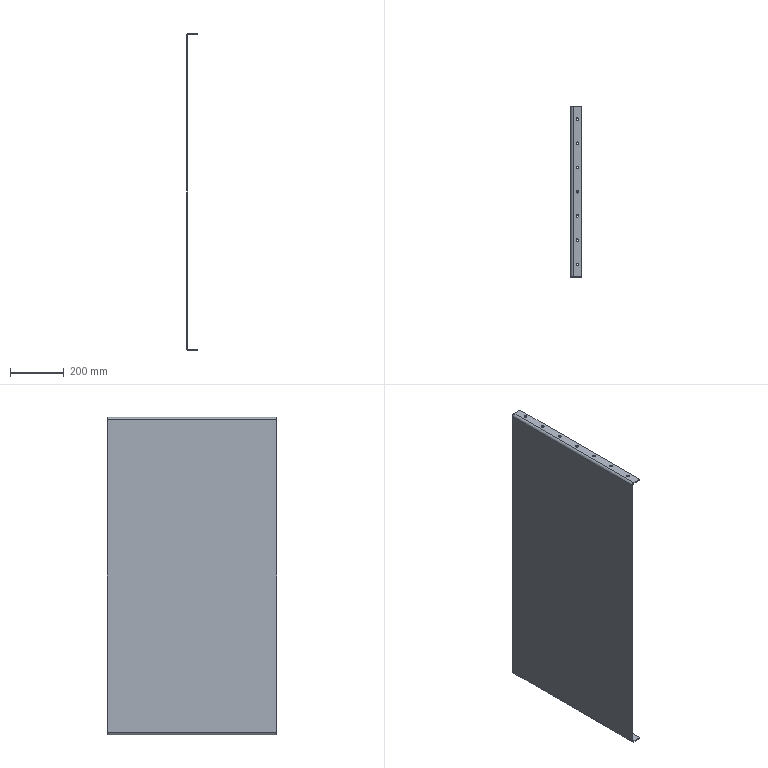Part | SolidWorks | features EdgeFlange 1, FlatPattern 1, HoleWzd 1, ICE 1, LPattern 1, SMBaseFlange 1, SheetMetal 1 | 1 solid | 50 faces | box 40 x 630 x 1180 mm | volume 3135499 mm3 | cylinder 32 | plane 18 | commonest cylinder face diameters 10 x30 18 x2
STEP:
#1=CARTESIAN_POINT('',(21.,40.,1180.));
#2=VERTEX_POINT('',#1);
#3=CARTESIAN_POINT('',(21.,50.,1180.));
#4=VERTEX_POINT('',#3);
#5=CARTESIAN_POINT('',(21.,45.,1180.));
#6=DIRECTION('',(0.,0.,-1.));
#7=DIRECTION('',(0.,1.,0.));
#8=AXIS2_PLACEMENT_3D('',#5,#6,#7);
#9=CIRCLE('',#8,5.);
#10=EDGE_CURVE('',#2,#4,#9,.T.);
#11=ORIENTED_EDGE('',*,*,#10,.F.);
#12=CARTESIAN_POINT('',(21.,40.,1176.));
#13=VERTEX_POINT('',#12);
#14=CARTESIAN_POINT('',(21.,40.,0.));
#15=DIRECTION('',(0.,0.,-1.));
#16=VECTOR('',#15,1000.);
#17=LINE('',#14,#16);
#18=EDGE_CURVE('',#2,#13,#17,.T.);
#19=ORIENTED_EDGE('',*,*,#18,.T.);
#20=CARTESIAN_POINT('',(21.,50.,1176.));
#21=VERTEX_POINT('',#20);
#22=CARTESIAN_POINT('',(21.,45.,1176.));
#23=DIRECTION('',(0.,0.,-1.));
#24=DIRECTION('',(-1.,0.,0.));
#25=AXIS2_PLACEMENT_3D('',#22,#23,#24);
#26=CIRCLE('',#25,5.);
#27=EDGE_CURVE('',#13,#21,#26,.T.);
#28=ORIENTED_EDGE('',*,*,#27,.T.);
#29=CARTESIAN_POINT('',(21.,50.,0.));
#30=DIRECTION('',(0.,0.,-1.));
#31=VECTOR('',#30,1000.);
#32=LINE('',#29,#31);
#33=EDGE_CURVE('',#4,#21,#32,.T.);
#34=ORIENTED_EDGE('',*,*,#33,.F.);
#35=EDGE_LOOP('',(#11,#19,#28,#34));
#36=FACE_OUTER_BOUND('',#35,.T.);
#37=CARTESIAN_POINT('',(21.,45.,0.));
#38=DIRECTION('',(0.,0.,-1.));
#39=DIRECTION('',(0.,1.,0.));
#40=AXIS2_PLACEMENT_3D('',#37,#38,#39);
#41=CYLINDRICAL_SURFACE('',#40,5.);
#42=ADVANCED_FACE('',(#36),#41,.F.);
#43=CARTESIAN_POINT('',(21.,130.,1180.));
#44=VERTEX_POINT('',#43);
#45=CARTESIAN_POINT('',(21.,140.,1180.));
#46=VERTEX_POINT('',#45);
#47=CARTESIAN_POINT('',(21.,135.,1180.));
#48=DIRECTION('',(0.,0.,-1.));
#49=DIRECTION('',(0.,1.,0.));
#50=AXIS2_PLACEMENT_3D('',#47,#48,#49);
#51=CIRCLE('',#50,5.);
#52=EDGE_CURVE('',#44,#46,#51,.T.);
#53=ORIENTED_EDGE('',*,*,#52,.F.);
#54=CARTESIAN_POINT('',(21.,130.,1176.));
#55=VERTEX_POINT('',#54);
#56=CARTESIAN_POINT('',(21.,130.,0.));
#57=DIRECTION('',(0.,0.,-1.));
#58=VECTOR('',#57,1000.);
#59=LINE('',#56,#58);
#60=EDGE_CURVE('',#44,#55,#59,.T.);
#61=ORIENTED_EDGE('',*,*,#60,.T.);
#62=CARTESIAN_POINT('',(21.,140.,1176.));
#63=VERTEX_POINT('',#62);
#64=CARTESIAN_POINT('',(21.,135.,1176.));
#65=DIRECTION('',(0.,0.,-1.));
#66=DIRECTION('',(-1.,0.,0.));
#67=AXIS2_PLACEMENT_3D('',#64,#65,#66);
#68=CIRCLE('',#67,5.);
#69=EDGE_CURVE('',#55,#63,#68,.T.);
#70=ORIENTED_EDGE('',*,*,#69,.T.);
#71=CARTESIAN_POINT('',(21.,140.,0.));
#72=DIRECTION('',(0.,0.,-1.));
#73=VECTOR('',#72,1000.);
#74=LINE('',#71,#73);
#75=EDGE_CURVE('',#46,#63,#74,.T.);
#76=ORIENTED_EDGE('',*,*,#75,.F.);
#77=EDGE_LOOP('',(#53,#61,#70,#76));
#78=FACE_OUTER_BOUND('',#77,.T.);
#79=CARTESIAN_POINT('',(21.,135.,0.));
#80=DIRECTION('',(0.,0.,-1.));
#81=DIRECTION('',(0.,1.,0.));
#82=AXIS2_PLACEMENT_3D('',#79,#80,#81);
#83=CYLINDRICAL_SURFACE('',#82,5.);
#84=ADVANCED_FACE('',(#78),#83,.F.);
#85=CARTESIAN_POINT('',(21.,220.,1180.));
#86=VERTEX_POINT('',#85);
#87=CARTESIAN_POINT('',(21.,230.,1180.));
#88=VERTEX_POINT('',#87);
#89=CARTESIAN_POINT('',(21.,225.,1180.));
#90=DIRECTION('',(0.,0.,-1.));
#91=DIRECTION('',(0.,1.,0.));
#92=AXIS2_PLACEMENT_3D('',#89,#90,#91);
#93=CIRCLE('',#92,5.);
#94=EDGE_CURVE('',#86,#88,#93,.T.);
#95=ORIENTED_EDGE('',*,*,#94,.F.);
#96=CARTESIAN_POINT('',(21.,220.,1176.));
#97=VERTEX_POINT('',#96);
#98=CARTESIAN_POINT('',(21.,220.,0.));
#99=DIRECTION('',(0.,0.,-1.));
#100=VECTOR('',#99,1000.);
#101=LINE('',#98,#100);
#102=EDGE_CURVE('',#86,#97,#101,.T.);
#103=ORIENTED_EDGE('',*,*,#102,.T.);
#104=CARTESIAN_POINT('',(21.,230.,1176.));
#105=VERTEX_POINT('',#104);
#106=CARTESIAN_POINT('',(21.,225.,1176.));
#107=DIRECTION('',(0.,0.,-1.));
#108=DIRECTION('',(-1.,0.,0.));
#109=AXIS2_PLACEMENT_3D('',#106,#107,#108);
#110=CIRCLE('',#109,5.);
#111=EDGE_CURVE('',#97,#105,#110,.T.);
#112=ORIENTED_EDGE('',*,*,#111,.T.);
#113=CARTESIAN_POINT('',(21.,230.,0.));
#114=DIRECTION('',(0.,0.,-1.));
#115=VECTOR('',#114,1000.);
#116=LINE('',#113,#115);
#117=EDGE_CURVE('',#88,#105,#116,.T.);
#118=ORIENTED_EDGE('',*,*,#117,.F.);
#119=EDGE_LOOP('',(#95,#103,#112,#118));
#120=FACE_OUTER_BOUND('',#119,.T.);
#121=CARTESIAN_POINT('',(21.,225.,0.));
#122=DIRECTION('',(0.,0.,-1.));
#123=DIRECTION('',(0.,1.,0.));
#124=AXIS2_PLACEMENT_3D('',#121,#122,#123);
#125=CYLINDRICAL_SURFACE('',#124,5.);
#126=ADVANCED_FACE('',(#120),#125,.F.);
#127=CARTESIAN_POINT('',(21.,310.,1180.));
#128=VERTEX_POINT('',#127);
#129=CARTESIAN_POINT('',(21.,320.,1180.));
#130=VERTEX_POINT('',#129);
#131=CARTESIAN_POINT('',(21.,315.,1180.));
#132=DIRECTION('',(0.,0.,-1.));
#133=DIRECTION('',(0.,1.,0.));
#134=AXIS2_PLACEMENT_3D('',#131,#132,#133);
#135=CIRCLE('',#134,5.);
#136=EDGE_CURVE('',#128,#130,#135,.T.);
#137=ORIENTED_EDGE('',*,*,#136,.F.);
#138=CARTESIAN_POINT('',(21.,310.,1176.));
#139=VERTEX_POINT('',#138);
#140=CARTESIAN_POINT('',(21.,310.,0.));
#141=DIRECTION('',(0.,0.,-1.));
#142=VECTOR('',#141,1000.);
#143=LINE('',#140,#142);
#144=EDGE_CURVE('',#128,#139,#143,.T.);
#145=ORIENTED_EDGE('',*,*,#144,.T.);
#146=CARTESIAN_POINT('',(21.,320.,1176.));
#147=VERTEX_POINT('',#146);
#148=CARTESIAN_POINT('',(21.,315.,1176.));
#149=DIRECTION('',(0.,0.,-1.));
#150=DIRECTION('',(-1.,0.,0.));
#151=AXIS2_PLACEMENT_3D('',#148,#149,#150);
#152=CIRCLE('',#151,5.);
#153=EDGE_CURVE('',#139,#147,#152,.T.);
#154=ORIENTED_EDGE('',*,*,#153,.T.);
#155=CARTESIAN_POINT('',(21.,320.,0.));
#156=DIRECTION('',(0.,0.,-1.));
#157=VECTOR('',#156,1000.);
#158=LINE('',#155,#157);
#159=EDGE_CURVE('',#130,#147,#158,.T.);
#160=ORIENTED_EDGE('',*,*,#159,.F.);
#161=EDGE_LOOP('',(#137,#145,#154,#160));
#162=FACE_OUTER_BOUND('',#161,.T.);
#163=CARTESIAN_POINT('',(21.,315.,0.));
#164=DIRECTION('',(0.,0.,-1.));
#165=DIRECTION('',(0.,1.,0.));
#166=AXIS2_PLACEMENT_3D('',#163,#164,#165);
#167=CYLINDRICAL_SURFACE('',#166,5.);
#168=ADVANCED_FACE('',(#162),#167,.F.);
#169=CARTESIAN_POINT('',(21.,400.,1180.));
#170=VERTEX_POINT('',#169);
#171=CARTESIAN_POINT('',(21.,410.,1180.));
#172=VERTEX_POINT('',#171);
#173=CARTESIAN_POINT('',(21.,405.,1180.));
#174=DIRECTION('',(0.,0.,-1.));
#175=DIRECTION('',(0.,1.,0.));
#176=AXIS2_PLACEMENT_3D('',#173,#174,#175);
#177=CIRCLE('',#176,5.);
#178=EDGE_CURVE('',#170,#172,#177,.T.);
#179=ORIENTED_EDGE('',*,*,#178,.F.);
#180=CARTESIAN_POINT('',(21.,400.,1176.));
#181=VERTEX_POINT('',#180);
#182=CARTESIAN_POINT('',(21.,400.,0.));
#183=DIRECTION('',(0.,0.,-1.));
#184=VECTOR('',#183,1000.);
#185=LINE('',#182,#184);
#186=EDGE_CURVE('',#170,#181,#185,.T.);
#187=ORIENTED_EDGE('',*,*,#186,.T.);
#188=CARTESIAN_POINT('',(21.,410.,1176.));
#189=VERTEX_POINT('',#188);
#190=CARTESIAN_POINT('',(21.,405.,1176.));
#191=DIRECTION('',(0.,0.,-1.));
#192=DIRECTION('',(-1.,0.,0.));
#193=AXIS2_PLACEMENT_3D('',#190,#191,#192);
#194=CIRCLE('',#193,5.);
#195=EDGE_CURVE('',#181,#189,#194,.T.);
#196=ORIENTED_EDGE('',*,*,#195,.T.);
#197=CARTESIAN_POINT('',(21.,410.,0.));
#198=DIRECTION('',(0.,0.,-1.));
#199=VECTOR('',#198,1000.);
#200=LINE('',#197,#199);
#201=EDGE_CURVE('',#172,#189,#200,.T.);
#202=ORIENTED_EDGE('',*,*,#201,.F.);
#203=EDGE_LOOP('',(#179,#187,#196,#202));
#204=FACE_OUTER_BOUND('',#203,.T.);
#205=CARTESIAN_POINT('',(21.,405.,0.));
#206=DIRECTION('',(0.,0.,-1.));
#207=DIRECTION('',(0.,1.,0.));
#208=AXIS2_PLACEMENT_3D('',#205,#206,#207);
#209=CYLINDRICAL_SURFACE('',#208,5.);
#210=ADVANCED_FACE('',(#204),#209,.F.);
#211=CARTESIAN_POINT('',(21.,490.,1180.));
#212=VERTEX_POINT('',#211);
#213=CARTESIAN_POINT('',(21.,500.,1180.));
#214=VERTEX_POINT('',#213);
#215=CARTESIAN_POINT('',(21.,495.,1180.));
#216=DIRECTION('',(0.,0.,-1.));
#217=DIRECTION('',(0.,1.,0.));
#218=AXIS2_PLACEMENT_3D('',#215,#216,#217);
#219=CIRCLE('',#218,5.);
#220=EDGE_CURVE('',#212,#214,#219,.T.);
#221=ORIENTED_EDGE('',*,*,#220,.F.);
#222=CARTESIAN_POINT('',(21.,490.,1176.));
#223=VERTEX_POINT('',#222);
#224=CARTESIAN_POINT('',(21.,490.,0.));
#225=DIRECTION('',(0.,0.,-1.));
#226=VECTOR('',#225,1000.);
#227=LINE('',#224,#226);
#228=EDGE_CURVE('',#212,#223,#227,.T.);
#229=ORIENTED_EDGE('',*,*,#228,.T.);
#230=CARTESIAN_POINT('',(21.,500.,1176.));
#231=VERTEX_POINT('',#230);
#232=CARTESIAN_POINT('',(21.,495.,1176.));
#233=DIRECTION('',(0.,0.,-1.));
#234=DIRECTION('',(-1.,0.,0.));
#235=AXIS2_PLACEMENT_3D('',#232,#233,#234);
#236=CIRCLE('',#235,5.);
#237=EDGE_CURVE('',#223,#231,#236,.T.);
#238=ORIENTED_EDGE('',*,*,#237,.T.);
#239=CARTESIAN_POINT('',(21.,500.,0.));
#240=DIRECTION('',(0.,0.,-1.));
#241=VECTOR('',#240,1000.);
#242=LINE('',#239,#241);
#243=EDGE_CURVE('',#214,#231,#242,.T.);
#244=ORIENTED_EDGE('',*,*,#243,.F.);
#245=EDGE_LOOP('',(#221,#229,#238,#244));
#246=FACE_OUTER_BOUND('',#245,.T.);
#247=CARTESIAN_POINT('',(21.,495.,0.));
#248=DIRECTION('',(0.,0.,-1.));
#249=DIRECTION('',(0.,1.,0.));
#250=AXIS2_PLACEMENT_3D('',#247,#248,#249);
#251=CYLINDRICAL_SURFACE('',#250,5.);
#252=ADVANCED_FACE('',(#246),#251,.F.);
#253=CARTESIAN_POINT('',(21.,50.,4.));
#254=VERTEX_POINT('',#253);
#255=CARTESIAN_POINT('',(21.,40.,4.));
#256=VERTEX_POINT('',#255);
#257=CARTESIAN_POINT('',(21.,45.,4.));
#258=DIRECTION('',(0.,0.,1.));
#259=DIRECTION('',(1.,0.,0.));
#260=AXIS2_PLACEMENT_3D('',#257,#258,#259);
#261=CIRCLE('',#260,5.);
#262=EDGE_CURVE('',#254,#256,#261,.T.);
#263=ORIENTED_EDGE('',*,*,#262,.T.);
#264=CARTESIAN_POINT('',(21.,40.,0.));
#265=VERTEX_POINT('',#264);
#266=CARTESIAN_POINT('',(21.,40.,0.));
#267=DIRECTION('',(0.,0.,-1.));
#268=VECTOR('',#267,1000.);
#269=LINE('',#266,#268);
#270=EDGE_CURVE('',#256,#265,#269,.T.);
#271=ORIENTED_EDGE('',*,*,#270,.T.);
#272=CARTESIAN_POINT('',(21.,50.,0.));
#273=VERTEX_POINT('',#272);
#274=CARTESIAN_POINT('',(21.,45.,0.));
#275=DIRECTION('',(0.,0.,-1.));
#276=DIRECTION('',(0.,1.,0.));
#277=AXIS2_PLACEMENT_3D('',#274,#275,#276);
#278=CIRCLE('',#277,5.);
#279=EDGE_CURVE('',#265,#273,#278,.T.);
#280=ORIENTED_EDGE('',*,*,#279,.T.);
#281=CARTESIAN_POINT('',(21.,50.,0.));
#282=DIRECTION('',(0.,0.,-1.));
#283=VECTOR('',#282,1000.);
#284=LINE('',#281,#283);
#285=EDGE_CURVE('',#254,#273,#284,.T.);
#286=ORIENTED_EDGE('',*,*,#285,.F.);
#287=EDGE_LOOP('',(#263,#271,#280,#286));
#288=FACE_OUTER_BOUND('',#287,.T.);
#289=CARTESIAN_POINT('',(21.,45.,0.));
#290=DIRECTION('',(0.,0.,-1.));
#291=DIRECTION('',(0.,1.,0.));
#292=AXIS2_PLACEMENT_3D('',#289,#290,#291);
#293=CYLINDRICAL_SURFACE('',#292,5.);
#294=ADVANCED_FACE('',(#288),#293,.F.);
#295=CARTESIAN_POINT('',(21.,140.,4.));
#296=VERTEX_POINT('',#295);
#297=CARTESIAN_POINT('',(21.,130.,4.));
#298=VERTEX_POINT('',#297);
#299=CARTESIAN_POINT('',(21.,135.,4.));
#300=DIRECTION('',(0.,0.,1.));
#301=DIRECTION('',(1.,0.,0.));
#302=AXIS2_PLACEMENT_3D('',#299,#300,#301);
#303=CIRCLE('',#302,5.);
#304=EDGE_CURVE('',#296,#298,#303,.T.);
#305=ORIENTED_EDGE('',*,*,#304,.T.);
#306=CARTESIAN_POINT('',(21.,130.,0.));
#307=VERTEX_POINT('',#306);
#308=CARTESIAN_POINT('',(21.,130.,0.));
#309=DIRECTION('',(0.,0.,-1.));
#310=VECTOR('',#309,1000.);
#311=LINE('',#308,#310);
#312=EDGE_CURVE('',#298,#307,#311,.T.);
#313=ORIENTED_EDGE('',*,*,#312,.T.);
#314=CARTESIAN_POINT('',(21.,140.,0.));
#315=VERTEX_POINT('',#314);
#316=CARTESIAN_POINT('',(21.,135.,0.));
#317=DIRECTION('',(0.,0.,-1.));
#318=DIRECTION('',(0.,1.,0.));
#319=AXIS2_PLACEMENT_3D('',#316,#317,#318);
#320=CIRCLE('',#319,5.);
#321=EDGE_CURVE('',#307,#315,#320,.T.);
#322=ORIENTED_EDGE('',*,*,#321,.T.);
#323=CARTESIAN_POINT('',(21.,140.,0.));
#324=DIRECTION('',(0.,0.,-1.));
#325=VECTOR('',#324,1000.);
#326=LINE('',#323,#325);
#327=EDGE_CURVE('',#296,#315,#326,.T.);
#328=ORIENTED_EDGE('',*,*,#327,.F.);
#329=EDGE_LOOP('',(#305,#313,#322,#328));
#330=FACE_OUTER_BOUND('',#329,.T.);
#331=CARTESIAN_POINT('',(21.,135.,0.));
#332=DIRECTION('',(0.,0.,-1.));
#333=DIRECTION('',(0.,1.,0.));
#334=AXIS2_PLACEMENT_3D('',#331,#332,#333);
#335=CYLINDRICAL_SURFACE('',#334,5.);
#336=ADVANCED_FACE('',(#330),#335,.F.);
#337=CARTESIAN_POINT('',(21.,230.,4.));
#338=VERTEX_POINT('',#337);
#339=CARTESIAN_POINT('',(21.,220.,4.));
#340=VERTEX_POINT('',#339);
#341=CARTESIAN_POINT('',(21.,225.,4.));
#342=DIRECTION('',(0.,0.,1.));
#343=DIRECTION('',(1.,0.,0.));
#344=AXIS2_PLACEMENT_3D('',#341,#342,#343);
#345=CIRCLE('',#344,5.);
#346=EDGE_CURVE('',#338,#340,#345,.T.);
#347=ORIENTED_EDGE('',*,*,#346,.T.);
#348=CARTESIAN_POINT('',(21.,220.,0.));
#349=VERTEX_POINT('',#348);
#350=CARTESIAN_POINT('',(21.,220.,0.));
#351=DIRECTION('',(0.,0.,-1.));
#352=VECTOR('',#351,1000.);
#353=LINE('',#350,#352);
#354=EDGE_CURVE('',#340,#349,#353,.T.);
#355=ORIENTED_EDGE('',*,*,#354,.T.);
#356=CARTESIAN_POINT('',(21.,230.,0.));
#357=VERTEX_POINT('',#356);
#358=CARTESIAN_POINT('',(21.,225.,0.));
#359=DIRECTION('',(0.,0.,-1.));
#360=DIRECTION('',(0.,1.,0.));
#361=AXIS2_PLACEMENT_3D('',#358,#359,#360);
#362=CIRCLE('',#361,5.);
#363=EDGE_CURVE('',#349,#357,#362,.T.);
#364=ORIENTED_EDGE('',*,*,#363,.T.);
#365=CARTESIAN_POINT('',(21.,230.,0.));
#366=DIRECTION('',(0.,0.,-1.));
#367=VECTOR('',#366,1000.);
#368=LINE('',#365,#367);
#369=EDGE_CURVE('',#338,#357,#368,.T.);
#370=ORIENTED_EDGE('',*,*,#369,.F.);
#371=EDGE_LOOP('',(#347,#355,#364,#370));
#372=FACE_OUTER_BOUND('',#371,.T.);
#373=CARTESIAN_POINT('',(21.,225.,0.));
#374=DIRECTION('',(0.,0.,-1.));
#375=DIRECTION('',(0.,1.,0.));
#376=AXIS2_PLACEMENT_3D('',#373,#374,#375);
#377=CYLINDRICAL_SURFACE('',#376,5.);
#378=ADVANCED_FACE('',(#372),#377,.F.);
#379=CARTESIAN_POINT('',(21.,320.,4.));
#380=VERTEX_POINT('',#379);
#381=CARTESIAN_POINT('',(21.,310.,4.));
#382=VERTEX_POINT('',#381);
#383=CARTESIAN_POINT('',(21.,315.,4.));
#384=DIRECTION('',(0.,0.,1.));
#385=DIRECTION('',(1.,0.,0.));
#386=AXIS2_PLACEMENT_3D('',#383,#384,#385);
#387=CIRCLE('',#386,5.);
#388=EDGE_CURVE('',#380,#382,#387,.T.);
#389=ORIENTED_EDGE('',*,*,#388,.T.);
#390=CARTESIAN_POINT('',(21.,310.,0.));
#391=VERTEX_POINT('',#390);
#392=CARTESIAN_POINT('',(21.,310.,0.));
#393=DIRECTION('',(0.,0.,-1.));
#394=VECTOR('',#393,1000.);
#395=LINE('',#392,#394);
#396=EDGE_CURVE('',#382,#391,#395,.T.);
#397=ORIENTED_EDGE('',*,*,#396,.T.);
#398=CARTESIAN_POINT('',(21.,320.,0.));
#399=VERTEX_POINT('',#398);
#400=CARTESIAN_POINT('',(21.,315.,0.));
#401=DIRECTION('',(0.,0.,-1.));
#402=DIRECTION('',(0.,1.,0.));
#403=AXIS2_PLACEMENT_3D('',#400,#401,#402);
#404=CIRCLE('',#403,5.);
#405=EDGE_CURVE('',#391,#399,#404,.T.);
#406=ORIENTED_EDGE('',*,*,#405,.T.);
#407=CARTESIAN_POINT('',(21.,320.,0.));
#408=DIRECTION('',(0.,0.,-1.));
#409=VECTOR('',#408,1000.);
#410=LINE('',#407,#409);
#411=EDGE_CURVE('',#380,#399,#410,.T.);
#412=ORIENTED_EDGE('',*,*,#411,.F.);
#413=EDGE_LOOP('',(#389,#397,#406,#412));
#414=FACE_OUTER_BOUND('',#413,.T.);
#415=CARTESIAN_POINT('',(21.,315.,0.));
#416=DIRECTION('',(0.,0.,-1.));
#417=DIRECTION('',(0.,1.,0.));
#418=AXIS2_PLACEMENT_3D('',#415,#416,#417);
#419=CYLINDRICAL_SURFACE('',#418,5.);
#420=ADVANCED_FACE('',(#414),#419,.F.);
#421=CARTESIAN_POINT('',(21.,410.,4.));
#422=VERTEX_POINT('',#421);
#423=CARTESIAN_POINT('',(21.,400.,4.));
#424=VERTEX_POINT('',#423);
#425=CARTESIAN_POINT('',(21.,405.,4.));
#426=DIRECTION('',(0.,0.,1.));
#427=DIRECTION('',(1.,0.,0.));
#428=AXIS2_PLACEMENT_3D('',#425,#426,#427);
#429=CIRCLE('',#428,5.);
#430=EDGE_CURVE('',#422,#424,#429,.T.);
#431=ORIENTED_EDGE('',*,*,#430,.T.);
#432=CARTESIAN_POINT('',(21.,400.,0.));
#433=VERTEX_POINT('',#432);
#434=CARTESIAN_POINT('',(21.,400.,0.));
#435=DIRECTION('',(0.,0.,-1.));
#436=VECTOR('',#435,1000.);
#437=LINE('',#434,#436);
#438=EDGE_CURVE('',#424,#433,#437,.T.);
#439=ORIENTED_EDGE('',*,*,#438,.T.);
#440=CARTESIAN_POINT('',(21.,410.,0.));
#441=VERTEX_POINT('',#440);
#442=CARTESIAN_POINT('',(21.,405.,0.));
#443=DIRECTION('',(0.,0.,-1.));
#444=DIRECTION('',(0.,1.,0.));
#445=AXIS2_PLACEMENT_3D('',#442,#443,#444);
#446=CIRCLE('',#445,5.);
#447=EDGE_CURVE('',#433,#441,#446,.T.);
#448=ORIENTED_EDGE('',*,*,#447,.T.);
#449=CARTESIAN_POINT('',(21.,410.,0.));
#450=DIRECTION('',(0.,0.,-1.));
#451=VECTOR('',#450,1000.);
#452=LINE('',#449,#451);
#453=EDGE_CURVE('',#422,#441,#452,.T.);
#454=ORIENTED_EDGE('',*,*,#453,.F.);
#455=EDGE_LOOP('',(#431,#439,#448,#454));
#456=FACE_OUTER_BOUND('',#455,.T.);
#457=CARTESIAN_POINT('',(21.,405.,0.));
#458=DIRECTION('',(0.,0.,-1.));
#459=DIRECTION('',(0.,1.,0.));
#460=AXIS2_PLACEMENT_3D('',#457,#458,#459);
#461=CYLINDRICAL_SURFACE('',#460,5.);
#462=ADVANCED_FACE('',(#456),#461,.F.);
#463=CARTESIAN_POINT('',(21.,500.,4.));
#464=VERTEX_POINT('',#463);
#465=CARTESIAN_POINT('',(21.,490.,4.));
#466=VERTEX_POINT('',#465);
#467=CARTESIAN_POINT('',(21.,495.,4.));
#468=DIRECTION('',(0.,0.,1.));
#469=DIRECTION('',(1.,0.,0.));
#470=AXIS2_PLACEMENT_3D('',#467,#468,#469);
#471=CIRCLE('',#470,5.);
#472=EDGE_CURVE('',#464,#466,#471,.T.);
#473=ORIENTED_EDGE('',*,*,#472,.T.);
#474=CARTESIAN_POINT('',(21.,490.,0.));
#475=VERTEX_POINT('',#474);
#476=CARTESIAN_POINT('',(21.,490.,0.));
#477=DIRECTION('',(0.,0.,-1.));
#478=VECTOR('',#477,1000.);
#479=LINE('',#476,#478);
#480=EDGE_CURVE('',#466,#475,#479,.T.);
#481=ORIENTED_EDGE('',*,*,#480,.T.);
#482=CARTESIAN_POINT('',(21.,500.,0.));
#483=VERTEX_POINT('',#482);
#484=CARTESIAN_POINT('',(21.,495.,0.));
#485=DIRECTION('',(0.,0.,-1.));
#486=DIRECTION('',(0.,1.,0.));
#487=AXIS2_PLACEMENT_3D('',#484,#485,#486);
#488=CIRCLE('',#487,5.);
#489=EDGE_CURVE('',#475,#483,#488,.T.);
#490=ORIENTED_EDGE('',*,*,#489,.T.);
#491=CARTESIAN_POINT('',(21.,500.,0.));
#492=DIRECTION('',(0.,0.,-1.));
#493=VECTOR('',#492,1000.);
#494=LINE('',#491,#493);
#495=EDGE_CURVE('',#464,#483,#494,.T.);
#496=ORIENTED_EDGE('',*,*,#495,.F.);
#497=EDGE_LOOP('',(#473,#481,#490,#496));
#498=FACE_OUTER_BOUND('',#497,.T.);
#499=CARTESIAN_POINT('',(21.,495.,0.));
#500=DIRECTION('',(0.,0.,-1.));
#501=DIRECTION('',(0.,1.,0.));
#502=AXIS2_PLACEMENT_3D('',#499,#500,#501);
#503=CYLINDRICAL_SURFACE('',#502,5.);
#504=ADVANCED_FACE('',(#498),#503,.F.);
#505=CARTESIAN_POINT('',(21.,590.,4.));
#506=VERTEX_POINT('',#505);
#507=CARTESIAN_POINT('',(21.,580.,4.));
#508=VERTEX_POINT('',#507);
#509=CARTESIAN_POINT('',(21.,585.,4.));
#510=DIRECTION('',(0.,0.,1.));
#511=DIRECTION('',(1.,0.,0.));
#512=AXIS2_PLACEMENT_3D('',#509,#510,#511);
#513=CIRCLE('',#512,5.);
#514=EDGE_CURVE('',#506,#508,#513,.T.);
#515=ORIENTED_EDGE('',*,*,#514,.T.);
#516=CARTESIAN_POINT('',(21.,580.,0.));
#517=VERTEX_POINT('',#516);
#518=CARTESIAN_POINT('',(21.,580.,0.));
#519=DIRECTION('',(0.,0.,-1.));
#520=VECTOR('',#519,1000.);
#521=LINE('',#518,#520);
#522=EDGE_CURVE('',#508,#517,#521,.T.);
#523=ORIENTED_EDGE('',*,*,#522,.T.);
#524=CARTESIAN_POINT('',(21.,590.,0.));
#525=VERTEX_POINT('',#524);
#526=CARTESIAN_POINT('',(21.,585.,0.));
#527=DIRECTION('',(0.,0.,-1.));
#528=DIRECTION('',(0.,1.,0.));
#529=AXIS2_PLACEMENT_3D('',#526,#527,#528);
#530=CIRCLE('',#529,5.);
#531=EDGE_CURVE('',#517,#525,#530,.T.);
#532=ORIENTED_EDGE('',*,*,#531,.T.);
#533=CARTESIAN_POINT('',(21.,590.,0.));
#534=DIRECTION('',(0.,0.,-1.));
#535=VECTOR('',#534,1000.);
#536=LINE('',#533,#535);
#537=EDGE_CURVE('',#506,#525,#536,.T.);
#538=ORIENTED_EDGE('',*,*,#537,.F.);
#539=EDGE_LOOP('',(#515,#523,#532,#538));
#540=FACE_OUTER_BOUND('',#539,.T.);
#541=CARTESIAN_POINT('',(21.,585.,0.));
#542=DIRECTION('',(0.,0.,-1.));
#543=DIRECTION('',(0.,1.,0.));
#544=AXIS2_PLACEMENT_3D('',#541,#542,#543);
#545=CYLINDRICAL_SURFACE('',#544,5.);
#546=ADVANCED_FACE('',(#540),#545,.F.);
#547=CARTESIAN_POINT('',(21.,580.,1180.));
#548=VERTEX_POINT('',#547);
#549=CARTESIAN_POINT('',(21.,590.,1180.));
#550=VERTEX_POINT('',#549);
#551=CARTESIAN_POINT('',(21.,585.,1180.));
#552=DIRECTION('',(0.,0.,-1.));
#553=DIRECTION('',(0.,1.,0.));
#554=AXIS2_PLACEMENT_3D('',#551,#552,#553);
#555=CIRCLE('',#554,5.);
#556=EDGE_CURVE('',#548,#550,#555,.T.);
#557=ORIENTED_EDGE('',*,*,#556,.F.);
#558=CARTESIAN_POINT('',(21.,580.,1176.));
#559=VERTEX_POINT('',#558);
#560=CARTESIAN_POINT('',(21.,580.,0.));
#561=DIRECTION('',(0.,0.,-1.));
#562=VECTOR('',#561,1000.);
#563=LINE('',#560,#562);
#564=EDGE_CURVE('',#548,#559,#563,.T.);
#565=ORIENTED_EDGE('',*,*,#564,.T.);
#566=CARTESIAN_POINT('',(21.,590.,1176.));
#567=VERTEX_POINT('',#566);
#568=CARTESIAN_POINT('',(21.,585.,1176.));
#569=DIRECTION('',(0.,0.,-1.));
#570=DIRECTION('',(-1.,0.,0.));
#571=AXIS2_PLACEMENT_3D('',#568,#569,#570);
#572=CIRCLE('',#571,5.);
#573=EDGE_CURVE('',#559,#567,#572,.T.);
#574=ORIENTED_EDGE('',*,*,#573,.T.);
#575=CARTESIAN_POINT('',(21.,590.,0.));
#576=DIRECTION('',(0.,0.,-1.));
#577=VECTOR('',#576,1000.);
#578=LINE('',#575,#577);
#579=EDGE_CURVE('',#550,#567,#578,.T.);
#580=ORIENTED_EDGE('',*,*,#579,.F.);
#581=EDGE_LOOP('',(#557,#565,#574,#580));
#582=FACE_OUTER_BOUND('',#581,.T.);
#583=CARTESIAN_POINT('',(21.,585.,0.));
#584=DIRECTION('',(0.,0.,-1.));
#585=DIRECTION('',(0.,1.,0.));
#586=AXIS2_PLACEMENT_3D('',#583,#584,#585);
#587=CYLINDRICAL_SURFACE('',#586,5.);
#588=ADVANCED_FACE('',(#582),#587,.F.);
#589=CARTESIAN_POINT('',(-4.,0.,1171.));
#590=VERTEX_POINT('',#589);
#591=CARTESIAN_POINT('',(-4.,630.,1171.));
#592=VERTEX_POINT('',#591);
#593=CARTESIAN_POINT('',(-4.,0.,1171.));
#594=DIRECTION('',(0.,1.,0.));
#595=VECTOR('',#594,1000.);
#596=LINE('',#593,#595);
#597=EDGE_CURVE('',#590,#592,#596,.T.);
#598=ORIENTED_EDGE('',*,*,#597,.T.);
#599=CARTESIAN_POINT('',(-4.,630.,9.));
#600=VERTEX_POINT('',#599);
#601=CARTESIAN_POINT('',(-4.,630.,1180.));
#602=DIRECTION('',(0.,0.,1.));
#603=VECTOR('',#602,1000.);
#604=LINE('',#601,#603);
#605=EDGE_CURVE('',#600,#592,#604,.T.);
#606=ORIENTED_EDGE('',*,*,#605,.F.);
#607=CARTESIAN_POINT('',(-4.,0.,9.));
#608=VERTEX_POINT('',#607);
#609=CARTESIAN_POINT('',(-4.,630.,9.));
#610=DIRECTION('',(0.,-1.,0.));
#611=VECTOR('',#610,1000.);
#612=LINE('',#609,#611);
#613=EDGE_CURVE('',#600,#608,#612,.T.);
#614=ORIENTED_EDGE('',*,*,#613,.T.);
#615=CARTESIAN_POINT('',(-4.,0.,1180.));
#616=DIRECTION('',(0.,0.,-1.));
#617=VECTOR('',#616,1000.);
#618=LINE('',#615,#617);
#619=EDGE_CURVE('',#590,#608,#618,.T.);
#620=ORIENTED_EDGE('',*,*,#619,.F.);
#621=EDGE_LOOP('',(#598,#606,#614,#620));
#622=FACE_OUTER_BOUND('',#621,.T.);
#623=CARTESIAN_POINT('',(-4.,0.,1180.));
#624=DIRECTION('',(1.,0.,0.));
#625=DIRECTION('',(0.,0.,-1.));
#626=AXIS2_PLACEMENT_3D('',#623,#624,#625);
#627=PLANE('',#626);
#628=ADVANCED_FACE('',(#622),#627,.F.);
#629=CARTESIAN_POINT('',(0.,630.,9.));
#630=VERTEX_POINT('',#629);
#631=CARTESIAN_POINT('',(0.,630.,1171.));
#632=VERTEX_POINT('',#631);
#633=CARTESIAN_POINT('',(0.,630.,1180.));
#634=DIRECTION('',(0.,0.,1.));
#635=VECTOR('',#634,1000.);
#636=LINE('',#633,#635);
#637=EDGE_CURVE('',#630,#632,#636,.T.);
#638=ORIENTED_EDGE('',*,*,#637,.T.);
#639=CARTESIAN_POINT('',(0.,0.,1171.));
#640=VERTEX_POINT('',#639);
#641=CARTESIAN_POINT('',(0.,0.,1171.));
#642=DIRECTION('',(0.,1.,0.));
#643=VECTOR('',#642,1000.);
#644=LINE('',#641,#643);
#645=EDGE_CURVE('',#640,#632,#644,.T.);
#646=ORIENTED_EDGE('',*,*,#645,.F.);
#647=CARTESIAN_POINT('',(0.,0.,9.));
#648=VERTEX_POINT('',#647);
#649=CARTESIAN_POINT('',(0.,0.,1180.));
#650=DIRECTION('',(0.,0.,-1.));
#651=VECTOR('',#650,1000.);
#652=LINE('',#649,#651);
#653=EDGE_CURVE('',#640,#648,#652,.T.);
#654=ORIENTED_EDGE('',*,*,#653,.T.);
#655=CARTESIAN_POINT('',(0.,630.,9.));
#656=DIRECTION('',(0.,-1.,0.));
#657=VECTOR('',#656,1000.);
#658=LINE('',#655,#657);
#659=EDGE_CURVE('',#630,#648,#658,.T.);
#660=ORIENTED_EDGE('',*,*,#659,.F.);
#661=EDGE_LOOP('',(#638,#646,#654,#660));
#662=FACE_OUTER_BOUND('',#661,.T.);
#663=CARTESIAN_POINT('',(0.,0.,1180.));
#664=DIRECTION('',(1.,0.,0.));
#665=DIRECTION('',(0.,0.,-1.));
#666=AXIS2_PLACEMENT_3D('',#663,#664,#665);
#667=PLANE('',#666);
#668=ADVANCED_FACE('',(#662),#667,.T.);
#669=ORIENTED_EDGE('',*,*,#653,.F.);
#670=CARTESIAN_POINT('',(0.,0.,1171.));
#671=DIRECTION('',(-1.,0.,0.));
#672=VECTOR('',#671,1000.);
#673=LINE('',#670,#672);
#674=EDGE_CURVE('',#640,#590,#673,.T.);
#675=ORIENTED_EDGE('',*,*,#674,.T.);
#676=ORIENTED_EDGE('',*,*,#619,.T.);
#677=CARTESIAN_POINT('',(0.,0.,9.));
#678=DIRECTION('',(-1.,0.,0.));
#679=VECTOR('',#678,1000.);
#680=LINE('',#677,#679);
#681=EDGE_CURVE('',#648,#608,#680,.T.);
#682=ORIENTED_EDGE('',*,*,#681,.F.);
#683=EDGE_LOOP('',(#669,#675,#676,#682));
#684=FACE_OUTER_BOUND('',#683,.T.);
#685=CARTESIAN_POINT('',(-4.,0.,1180.));
#686=DIRECTION('',(0.,-1.,0.));
#687=DIRECTION('',(0.,0.,-1.));
#688=AXIS2_PLACEMENT_3D('',#685,#686,#687);
#689=PLANE('',#688);
#690=ADVANCED_FACE('',(#684),#689,.T.);
#691=CARTESIAN_POINT('',(0.,630.,1171.));
#692=DIRECTION('',(-1.,0.,0.));
#693=VECTOR('',#692,1000.);
#694=LINE('',#691,#693);
#695=EDGE_CURVE('',#632,#592,#694,.T.);
#696=ORIENTED_EDGE('',*,*,#695,.F.);
#697=ORIENTED_EDGE('',*,*,#637,.F.);
#698=CARTESIAN_POINT('',(0.,630.,9.));
#699=DIRECTION('',(-1.,0.,0.));
#700=VECTOR('',#699,1000.);
#701=LINE('',#698,#700);
#702=EDGE_CURVE('',#630,#600,#701,.T.);
#703=ORIENTED_EDGE('',*,*,#702,.T.);
#704=ORIENTED_EDGE('',*,*,#605,.T.);
#705=EDGE_LOOP('',(#696,#697,#703,#704));
#706=FACE_OUTER_BOUND('',#705,.T.);
#707=CARTESIAN_POINT('',(-4.,630.,1180.));
#708=DIRECTION('',(0.,1.,0.));
#709=DIRECTION('',(0.,0.,1.));
#710=AXIS2_PLACEMENT_3D('',#707,#708,#709);
#711=PLANE('',#710);
#712=ADVANCED_FACE('',(#706),#711,.T.);
#713=CARTESIAN_POINT('',(5.,0.,4.));
#714=VERTEX_POINT('',#713);
#715=CARTESIAN_POINT('',(5.,0.,0.));
#716=VERTEX_POINT('',#715);
#717=CARTESIAN_POINT('',(5.,0.,0.));
#718=DIRECTION('',(0.,0.,-1.));
#719=VECTOR('',#718,1000.);
#720=LINE('',#717,#719);
#721=EDGE_CURVE('',#714,#716,#720,.T.);
#722=ORIENTED_EDGE('',*,*,#721,.F.);
#723=CARTESIAN_POINT('',(5.,0.,9.));
#724=DIRECTION('',(0.,-1.,0.));
#725=DIRECTION('',(0.,0.,1.));
#726=AXIS2_PLACEMENT_3D('',#723,#724,#725);
#727=CIRCLE('',#726,5.);
#728=EDGE_CURVE('',#648,#714,#727,.T.);
#729=ORIENTED_EDGE('',*,*,#728,.F.);
#730=ORIENTED_EDGE('',*,*,#681,.T.);
#731=CARTESIAN_POINT('',(5.,0.,9.));
#732=DIRECTION('',(0.,-1.,0.));
#733=DIRECTION('',(0.,0.,1.));
#734=AXIS2_PLACEMENT_3D('',#731,#732,#733);
#735=CIRCLE('',#734,9.);
#736=EDGE_CURVE('',#608,#716,#735,.T.);
#737=ORIENTED_EDGE('',*,*,#736,.T.);
#738=EDGE_LOOP('',(#722,#729,#730,#737));
#739=FACE_OUTER_BOUND('',#738,.T.);
#740=CARTESIAN_POINT('',(5.,0.,9.));
#741=DIRECTION('',(0.,-1.,0.));
#742=DIRECTION('',(0.,0.,-1.));
#743=AXIS2_PLACEMENT_3D('',#740,#741,#742);
#744=PLANE('',#743);
#745=ADVANCED_FACE('',(#739),#744,.T.);
#746=CARTESIAN_POINT('',(5.,630.,4.));
#747=VERTEX_POINT('',#746);
#748=CARTESIAN_POINT('',(5.,630.,9.));
#749=DIRECTION('',(0.,1.,0.));
#750=DIRECTION('',(0.,0.,1.));
#751=AXIS2_PLACEMENT_3D('',#748,#749,#750);
#752=CIRCLE('',#751,5.);
#753=EDGE_CURVE('',#747,#630,#752,.T.);
#754=ORIENTED_EDGE('',*,*,#753,.F.);
#755=CARTESIAN_POINT('',(5.,630.,0.));
#756=VERTEX_POINT('',#755);
#757=CARTESIAN_POINT('',(5.,630.,4.));
#758=DIRECTION('',(0.,0.,-1.));
#759=VECTOR('',#758,1000.);
#760=LINE('',#757,#759);
#761=EDGE_CURVE('',#747,#756,#760,.T.);
#762=ORIENTED_EDGE('',*,*,#761,.T.);
#763=CARTESIAN_POINT('',(5.,630.,9.));
#764=DIRECTION('',(0.,1.,0.));
#765=DIRECTION('',(0.,0.,1.));
#766=AXIS2_PLACEMENT_3D('',#763,#764,#765);
#767=CIRCLE('',#766,9.);
#768=EDGE_CURVE('',#756,#600,#767,.T.);
#769=ORIENTED_EDGE('',*,*,#768,.T.);
#770=ORIENTED_EDGE('',*,*,#702,.F.);
#771=EDGE_LOOP('',(#754,#762,#769,#770));
#772=FACE_OUTER_BOUND('',#771,.T.);
#773=CARTESIAN_POINT('',(5.,630.,9.));
#774=DIRECTION('',(0.,-1.,0.));
#775=DIRECTION('',(0.,0.,-1.));
#776=AXIS2_PLACEMENT_3D('',#773,#774,#775);
#777=PLANE('',#776);
#778=ADVANCED_FACE('',(#772),#777,.F.);
#779=ORIENTED_EDGE('',*,*,#613,.F.);
#780=ORIENTED_EDGE('',*,*,#768,.F.);
#781=CARTESIAN_POINT('',(5.,0.,0.));
#782=DIRECTION('',(0.,-1.,0.));
#783=VECTOR('',#782,1000.);
#784=LINE('',#781,#783);
#785=EDGE_CURVE('',#756,#716,#784,.T.);
#786=ORIENTED_EDGE('',*,*,#785,.T.);
#787=ORIENTED_EDGE('',*,*,#736,.F.);
#788=EDGE_LOOP('',(#779,#780,#786,#787));
#789=FACE_OUTER_BOUND('',#788,.T.);
#790=CARTESIAN_POINT('',(5.,630.,9.));
#791=DIRECTION('',(0.,1.,0.));
#792=DIRECTION('',(0.,0.,-1.));
#793=AXIS2_PLACEMENT_3D('',#790,#791,#792);
#794=CYLINDRICAL_SURFACE('',#793,9.);
#795=ADVANCED_FACE('',(#789),#794,.T.);
#796=ORIENTED_EDGE('',*,*,#659,.T.);
#797=ORIENTED_EDGE('',*,*,#728,.T.);
#798=CARTESIAN_POINT('',(5.,0.,4.));
#799=DIRECTION('',(0.,1.,0.));
#800=VECTOR('',#799,1000.);
#801=LINE('',#798,#800);
#802=EDGE_CURVE('',#714,#747,#801,.T.);
#803=ORIENTED_EDGE('',*,*,#802,.T.);
#804=ORIENTED_EDGE('',*,*,#753,.T.);
#805=EDGE_LOOP('',(#796,#797,#803,#804));
#806=FACE_OUTER_BOUND('',#805,.T.);
#807=CARTESIAN_POINT('',(5.,630.,9.));
#808=DIRECTION('',(0.,1.,0.));
#809=DIRECTION('',(0.,0.,-1.));
#810=AXIS2_PLACEMENT_3D('',#807,#808,#809);
#811=CYLINDRICAL_SURFACE('',#810,5.);
#812=ADVANCED_FACE('',(#806),#811,.F.);
#813=ORIENTED_EDGE('',*,*,#761,.F.);
#814=CARTESIAN_POINT('',(36.,630.,4.));
#815=VERTEX_POINT('',#814);
#816=CARTESIAN_POINT('',(36.,630.,4.));
#817=DIRECTION('',(1.,0.,0.));
#818=VECTOR('',#817,1000.);
#819=LINE('',#816,#818);
#820=EDGE_CURVE('',#747,#815,#819,.T.);
#821=ORIENTED_EDGE('',*,*,#820,.T.);
#822=CARTESIAN_POINT('',(36.,630.,0.));
#823=VERTEX_POINT('',#822);
#824=CARTESIAN_POINT('',(36.,630.,0.));
#825=DIRECTION('',(0.,0.,1.));
#826=VECTOR('',#825,1000.);
#827=LINE('',#824,#826);
#828=EDGE_CURVE('',#823,#815,#827,.T.);
#829=ORIENTED_EDGE('',*,*,#828,.F.);
#830=CARTESIAN_POINT('',(0.,630.,0.));
#831=DIRECTION('',(1.,0.,0.));
#832=VECTOR('',#831,1000.);
#833=LINE('',#830,#832);
#834=EDGE_CURVE('',#756,#823,#833,.T.);
#835=ORIENTED_EDGE('',*,*,#834,.F.);
#836=EDGE_LOOP('',(#813,#821,#829,#835));
#837=FACE_OUTER_BOUND('',#836,.T.);
#838=CARTESIAN_POINT('',(36.,630.,0.));
#839=DIRECTION('',(0.,-1.,0.));
#840=DIRECTION('',(0.,0.,-1.));
#841=AXIS2_PLACEMENT_3D('',#838,#839,#840);
#842=PLANE('',#841);
#843=ADVANCED_FACE('',(#837),#842,.F.);
#844=ORIENTED_EDGE('',*,*,#721,.T.);
#845=CARTESIAN_POINT('',(36.,0.,0.));
#846=VERTEX_POINT('',#845);
#847=CARTESIAN_POINT('',(0.,0.,0.));
#848=DIRECTION('',(-1.,0.,0.));
#849=VECTOR('',#848,1000.);
#850=LINE('',#847,#849);
#851=EDGE_CURVE('',#846,#716,#850,.T.);
#852=ORIENTED_EDGE('',*,*,#851,.F.);
#853=CARTESIAN_POINT('',(36.,0.,4.));
#854=VERTEX_POINT('',#853);
#855=CARTESIAN_POINT('',(36.,0.,0.));
#856=DIRECTION('',(0.,0.,1.));
#857=VECTOR('',#856,1000.);
#858=LINE('',#855,#857);
#859=EDGE_CURVE('',#846,#854,#858,.T.);
#860=ORIENTED_EDGE('',*,*,#859,.T.);
#861=CARTESIAN_POINT('',(0.,0.,4.));
#862=DIRECTION('',(-1.,0.,0.));
#863=VECTOR('',#862,1000.);
#864=LINE('',#861,#863);
#865=EDGE_CURVE('',#854,#714,#864,.T.);
#866=ORIENTED_EDGE('',*,*,#865,.T.);
#867=EDGE_LOOP('',(#844,#852,#860,#866));
#868=FACE_OUTER_BOUND('',#867,.T.);
#869=CARTESIAN_POINT('',(0.,0.,0.));
#870=DIRECTION('',(0.,1.,0.));
#871=DIRECTION('',(0.,0.,1.));
#872=AXIS2_PLACEMENT_3D('',#869,#870,#871);
#873=PLANE('',#872);
#874=ADVANCED_FACE('',(#868),#873,.F.);
#875=CARTESIAN_POINT('',(21.,495.,0.));
#876=DIRECTION('',(0.,0.,-1.));
#877=DIRECTION('',(0.,1.,0.));
#878=AXIS2_PLACEMENT_3D('',#875,#876,#877);
#879=CIRCLE('',#878,5.);
#880=EDGE_CURVE('',#483,#475,#879,.T.);
#881=ORIENTED_EDGE('',*,*,#880,.F.);
#882=ORIENTED_EDGE('',*,*,#489,.F.);
#883=EDGE_LOOP('',(#881,#882));
#884=FACE_BOUND('',#883,.T.);
#885=CARTESIAN_POINT('',(21.,585.,0.));
#886=DIRECTION('',(0.,0.,-1.));
#887=DIRECTION('',(0.,1.,0.));
#888=AXIS2_PLACEMENT_3D('',#885,#886,#887);
#889=CIRCLE('',#888,5.);
#890=EDGE_CURVE('',#525,#517,#889,.T.);
#891=ORIENTED_EDGE('',*,*,#890,.F.);
#892=ORIENTED_EDGE('',*,*,#531,.F.);
#893=EDGE_LOOP('',(#891,#892));
#894=FACE_BOUND('',#893,.T.);
#895=ORIENTED_EDGE('',*,*,#785,.F.);
#896=ORIENTED_EDGE('',*,*,#834,.T.);
#897=CARTESIAN_POINT('',(36.,630.,0.));
#898=DIRECTION('',(0.,-1.,0.));
#899=VECTOR('',#898,1000.);
#900=LINE('',#897,#899);
#901=EDGE_CURVE('',#823,#846,#900,.T.);
#902=ORIENTED_EDGE('',*,*,#901,.T.);
#903=ORIENTED_EDGE('',*,*,#851,.T.);
#904=EDGE_LOOP('',(#895,#896,#902,#903));
#905=FACE_OUTER_BOUND('',#904,.T.);
#906=CARTESIAN_POINT('',(21.,405.,0.));
#907=DIRECTION('',(0.,0.,-1.));
#908=DIRECTION('',(0.,1.,0.));
#909=AXIS2_PLACEMENT_3D('',#906,#907,#908);
#910=CIRCLE('',#909,5.);
#911=EDGE_CURVE('',#441,#433,#910,.T.);
#912=ORIENTED_EDGE('',*,*,#911,.F.);
#913=ORIENTED_EDGE('',*,*,#447,.F.);
#914=EDGE_LOOP('',(#912,#913));
#915=FACE_BOUND('',#914,.T.);
#916=CARTESIAN_POINT('',(21.,315.,0.));
#917=DIRECTION('',(0.,0.,-1.));
#918=DIRECTION('',(0.,1.,0.));
#919=AXIS2_PLACEMENT_3D('',#916,#917,#918);
#920=CIRCLE('',#919,5.);
#921=EDGE_CURVE('',#399,#391,#920,.T.);
#922=ORIENTED_EDGE('',*,*,#921,.F.);
#923=ORIENTED_EDGE('',*,*,#405,.F.);
#924=EDGE_LOOP('',(#922,#923));
#925=FACE_BOUND('',#924,.T.);
#926=CARTESIAN_POINT('',(21.,225.,0.));
#927=DIRECTION('',(0.,0.,-1.));
#928=DIRECTION('',(0.,1.,0.));
#929=AXIS2_PLACEMENT_3D('',#926,#927,#928);
#930=CIRCLE('',#929,5.);
#931=EDGE_CURVE('',#357,#349,#930,.T.);
#932=ORIENTED_EDGE('',*,*,#931,.F.);
#933=ORIENTED_EDGE('',*,*,#363,.F.);
#934=EDGE_LOOP('',(#932,#933));
#935=FACE_BOUND('',#934,.T.);
#936=CARTESIAN_POINT('',(21.,135.,0.));
#937=DIRECTION('',(0.,0.,-1.));
#938=DIRECTION('',(0.,1.,0.));
#939=AXIS2_PLACEMENT_3D('',#936,#937,#938);
#940=CIRCLE('',#939,5.);
#941=EDGE_CURVE('',#315,#307,#940,.T.);
#942=ORIENTED_EDGE('',*,*,#941,.F.);
#943=ORIENTED_EDGE('',*,*,#321,.F.);
#944=EDGE_LOOP('',(#942,#943));
#945=FACE_BOUND('',#944,.T.);
#946=CARTESIAN_POINT('',(21.,45.,0.));
#947=DIRECTION('',(0.,0.,-1.));
#948=DIRECTION('',(0.,1.,0.));
#949=AXIS2_PLACEMENT_3D('',#946,#947,#948);
#950=CIRCLE('',#949,5.);
#951=EDGE_CURVE('',#273,#265,#950,.T.);
#952=ORIENTED_EDGE('',*,*,#951,.F.);
#953=ORIENTED_EDGE('',*,*,#279,.F.);
#954=EDGE_LOOP('',(#952,#953));
#955=FACE_BOUND('',#954,.T.);
#956=CARTESIAN_POINT('',(0.,630.,0.));
#957=DIRECTION('',(0.,0.,1.));
#958=DIRECTION('',(1.,0.,0.));
#959=AXIS2_PLACEMENT_3D('',#956,#957,#958);
#960=PLANE('',#959);
#961=ADVANCED_FACE('',(#884,#894,#905,#915,#925,#935,#945,#955),#960,.F.);
#962=ORIENTED_EDGE('',*,*,#472,.F.);
#963=CARTESIAN_POINT('',(21.,495.,4.));
#964=DIRECTION('',(0.,0.,1.));
#965=DIRECTION('',(1.,0.,0.));
#966=AXIS2_PLACEMENT_3D('',#963,#964,#965);
#967=CIRCLE('',#966,5.);
#968=EDGE_CURVE('',#466,#464,#967,.T.);
#969=ORIENTED_EDGE('',*,*,#968,.F.);
#970=EDGE_LOOP('',(#962,#969));
#971=FACE_BOUND('',#970,.T.);
#972=ORIENTED_EDGE('',*,*,#514,.F.);
#973=CARTESIAN_POINT('',(21.,585.,4.));
#974=DIRECTION('',(0.,0.,1.));
#975=DIRECTION('',(1.,0.,0.));
#976=AXIS2_PLACEMENT_3D('',#973,#974,#975);
#977=CIRCLE('',#976,5.);
#978=EDGE_CURVE('',#508,#506,#977,.T.);
#979=ORIENTED_EDGE('',*,*,#978,.F.);
#980=EDGE_LOOP('',(#972,#979));
#981=FACE_BOUND('',#980,.T.);
#982=ORIENTED_EDGE('',*,*,#820,.F.);
#983=ORIENTED_EDGE('',*,*,#802,.F.);
#984=ORIENTED_EDGE('',*,*,#865,.F.);
#985=CARTESIAN_POINT('',(36.,0.,4.));
#986=DIRECTION('',(0.,-1.,0.));
#987=VECTOR('',#986,1000.);
#988=LINE('',#985,#987);
#989=EDGE_CURVE('',#815,#854,#988,.T.);
#990=ORIENTED_EDGE('',*,*,#989,.F.);
#991=EDGE_LOOP('',(#982,#983,#984,#990));
#992=FACE_OUTER_BOUND('',#991,.T.);
#993=ORIENTED_EDGE('',*,*,#430,.F.);
#994=CARTESIAN_POINT('',(21.,405.,4.));
#995=DIRECTION('',(0.,0.,1.));
#996=DIRECTION('',(1.,0.,0.));
#997=AXIS2_PLACEMENT_3D('',#994,#995,#996);
#998=CIRCLE('',#997,5.);
#999=EDGE_CURVE('',#424,#422,#998,.T.);
#1000=ORIENTED_EDGE('',*,*,#999,.F.);
#1001=EDGE_LOOP('',(#993,#1000));
#1002=FACE_BOUND('',#1001,.T.);
#1003=ORIENTED_EDGE('',*,*,#388,.F.);
#1004=CARTESIAN_POINT('',(21.,315.,4.));
#1005=DIRECTION('',(0.,0.,1.));
#1006=DIRECTION('',(1.,0.,0.));
#1007=AXIS2_PLACEMENT_3D('',#1004,#1005,#1006);
#1008=CIRCLE('',#1007,5.);
#1009=EDGE_CURVE('',#382,#380,#1008,.T.);
#1010=ORIENTED_EDGE('',*,*,#1009,.F.);
#1011=EDGE_LOOP('',(#1003,#1010));
#1012=FACE_BOUND('',#1011,.T.);
#1013=ORIENTED_EDGE('',*,*,#346,.F.);
#1014=CARTESIAN_POINT('',(21.,225.,4.));
#1015=DIRECTION('',(0.,0.,1.));
#1016=DIRECTION('',(1.,0.,0.));
#1017=AXIS2_PLACEMENT_3D('',#1014,#1015,#1016);
#1018=CIRCLE('',#1017,5.);
#1019=EDGE_CURVE('',#340,#338,#1018,.T.);
#1020=ORIENTED_EDGE('',*,*,#1019,.F.);
#1021=EDGE_LOOP('',(#1013,#1020));
#1022=FACE_BOUND('',#1021,.T.);
#1023=ORIENTED_EDGE('',*,*,#304,.F.);
#1024=CARTESIAN_POINT('',(21.,135.,4.));
#1025=DIRECTION('',(0.,0.,1.));
#1026=DIRECTION('',(1.,0.,0.));
#1027=AXIS2_PLACEMENT_3D('',#1024,#1025,#1026);
#1028=CIRCLE('',#1027,5.);
#1029=EDGE_CURVE('',#298,#296,#1028,.T.);
#1030=ORIENTED_EDGE('',*,*,#1029,.F.);
#1031=EDGE_LOOP('',(#1023,#1030));
#1032=FACE_BOUND('',#1031,.T.);
#1033=ORIENTED_EDGE('',*,*,#262,.F.);
#1034=CARTESIAN_POINT('',(21.,45.,4.));
#1035=DIRECTION('',(0.,0.,1.));
#1036=DIRECTION('',(1.,0.,0.));
#1037=AXIS2_PLACEMENT_3D('',#1034,#1035,#1036);
#1038=CIRCLE('',#1037,5.);
#1039=EDGE_CURVE('',#256,#254,#1038,.T.);
#1040=ORIENTED_EDGE('',*,*,#1039,.F.);
#1041=EDGE_LOOP('',(#1033,#1040));
#1042=FACE_BOUND('',#1041,.T.);
#1043=CARTESIAN_POINT('',(0.,630.,4.));
#1044=DIRECTION('',(0.,0.,1.));
#1045=DIRECTION('',(1.,0.,0.));
#1046=AXIS2_PLACEMENT_3D('',#1043,#1044,#1045);
#1047=PLANE('',#1046);
#1048=ADVANCED_FACE('',(#971,#981,#992,#1002,#1012,#1022,#1032,#1042),#1047,.T.);
#1049=ORIENTED_EDGE('',*,*,#989,.T.);
#1050=ORIENTED_EDGE('',*,*,#859,.F.);
#1051=ORIENTED_EDGE('',*,*,#901,.F.);
#1052=ORIENTED_EDGE('',*,*,#828,.T.);
#1053=EDGE_LOOP('',(#1049,#1050,#1051,#1052));
#1054=FACE_OUTER_BOUND('',#1053,.T.);
#1055=CARTESIAN_POINT('',(36.,0.,0.));
#1056=DIRECTION('',(-1.,0.,0.));
#1057=DIRECTION('',(0.,0.,1.));
#1058=AXIS2_PLACEMENT_3D('',#1055,#1056,#1057);
#1059=PLANE('',#1058);
#1060=ADVANCED_FACE('',(#1054),#1059,.F.);
#1061=CARTESIAN_POINT('',(5.,630.,1176.));
#1062=VERTEX_POINT('',#1061);
#1063=CARTESIAN_POINT('',(5.,630.,1180.));
#1064=VERTEX_POINT('',#1063);
#1065=CARTESIAN_POINT('',(5.,630.,1180.));
#1066=DIRECTION('',(0.,0.,1.));
#1067=VECTOR('',#1066,1000.);
#1068=LINE('',#1065,#1067);
#1069=EDGE_CURVE('',#1062,#1064,#1068,.T.);
#1070=ORIENTED_EDGE('',*,*,#1069,.F.);
#1071=CARTESIAN_POINT('',(5.,630.,1171.));
#1072=DIRECTION('',(0.,1.,0.));
#1073=DIRECTION('',(0.,0.,-1.));
#1074=AXIS2_PLACEMENT_3D('',#1071,#1072,#1073);
#1075=CIRCLE('',#1074,5.);
#1076=EDGE_CURVE('',#632,#1062,#1075,.T.);
#1077=ORIENTED_EDGE('',*,*,#1076,.F.);
#1078=ORIENTED_EDGE('',*,*,#695,.T.);
#1079=CARTESIAN_POINT('',(5.,630.,1171.));
#1080=DIRECTION('',(0.,1.,0.));
#1081=DIRECTION('',(0.,0.,-1.));
#1082=AXIS2_PLACEMENT_3D('',#1079,#1080,#1081);
#1083=CIRCLE('',#1082,9.);
#1084=EDGE_CURVE('',#592,#1064,#1083,.T.);
#1085=ORIENTED_EDGE('',*,*,#1084,.T.);
#1086=EDGE_LOOP('',(#1070,#1077,#1078,#1085));
#1087=FACE_OUTER_BOUND('',#1086,.T.);
#1088=CARTESIAN_POINT('',(5.,630.,1171.));
#1089=DIRECTION('',(0.,1.,0.));
#1090=DIRECTION('',(0.,0.,1.));
#1091=AXIS2_PLACEMENT_3D('',#1088,#1089,#1090);
#1092=PLANE('',#1091);
#1093=ADVANCED_FACE('',(#1087),#1092,.T.);
#1094=CARTESIAN_POINT('',(5.,0.,1176.));
#1095=VERTEX_POINT('',#1094);
#1096=CARTESIAN_POINT('',(5.,0.,1171.));
#1097=DIRECTION('',(0.,-1.,0.));
#1098=DIRECTION('',(0.,0.,-1.));
#1099=AXIS2_PLACEMENT_3D('',#1096,#1097,#1098);
#1100=CIRCLE('',#1099,5.);
#1101=EDGE_CURVE('',#1095,#640,#1100,.T.);
#1102=ORIENTED_EDGE('',*,*,#1101,.F.);
#1103=CARTESIAN_POINT('',(5.,0.,1180.));
#1104=VERTEX_POINT('',#1103);
#1105=CARTESIAN_POINT('',(5.,0.,1176.));
#1106=DIRECTION('',(0.,0.,1.));
#1107=VECTOR('',#1106,1000.);
#1108=LINE('',#1105,#1107);
#1109=EDGE_CURVE('',#1095,#1104,#1108,.T.);
#1110=ORIENTED_EDGE('',*,*,#1109,.T.);
#1111=CARTESIAN_POINT('',(5.,0.,1171.));
#1112=DIRECTION('',(0.,-1.,0.));
#1113=DIRECTION('',(0.,0.,-1.));
#1114=AXIS2_PLACEMENT_3D('',#1111,#1112,#1113);
#1115=CIRCLE('',#1114,9.);
#1116=EDGE_CURVE('',#1104,#590,#1115,.T.);
#1117=ORIENTED_EDGE('',*,*,#1116,.T.);
#1118=ORIENTED_EDGE('',*,*,#674,.F.);
#1119=EDGE_LOOP('',(#1102,#1110,#1117,#1118));
#1120=FACE_OUTER_BOUND('',#1119,.T.);
#1121=CARTESIAN_POINT('',(5.,0.,1171.));
#1122=DIRECTION('',(0.,1.,0.));
#1123=DIRECTION('',(0.,0.,1.));
#1124=AXIS2_PLACEMENT_3D('',#1121,#1122,#1123);
#1125=PLANE('',#1124);
#1126=ADVANCED_FACE('',(#1120),#1125,.F.);
#1127=ORIENTED_EDGE('',*,*,#597,.F.);
#1128=ORIENTED_EDGE('',*,*,#1116,.F.);
#1129=CARTESIAN_POINT('',(5.,630.,1180.));
#1130=DIRECTION('',(0.,1.,0.));
#1131=VECTOR('',#1130,1000.);
#1132=LINE('',#1129,#1131);
#1133=EDGE_CURVE('',#1104,#1064,#1132,.T.);
#1134=ORIENTED_EDGE('',*,*,#1133,.T.);
#1135=ORIENTED_EDGE('',*,*,#1084,.F.);
#1136=EDGE_LOOP('',(#1127,#1128,#1134,#1135));
#1137=FACE_OUTER_BOUND('',#1136,.T.);
#1138=CARTESIAN_POINT('',(5.,0.,1171.));
#1139=DIRECTION('',(0.,-1.,0.));
#1140=DIRECTION('',(0.,0.,1.));
#1141=AXIS2_PLACEMENT_3D('',#1138,#1139,#1140);
#1142=CYLINDRICAL_SURFACE('',#1141,9.);
#1143=ADVANCED_FACE('',(#1137),#1142,.T.);
#1144=ORIENTED_EDGE('',*,*,#645,.T.);
#1145=ORIENTED_EDGE('',*,*,#1076,.T.);
#1146=CARTESIAN_POINT('',(5.,630.,1176.));
#1147=DIRECTION('',(0.,-1.,0.));
#1148=VECTOR('',#1147,1000.);
#1149=LINE('',#1146,#1148);
#1150=EDGE_CURVE('',#1062,#1095,#1149,.T.);
#1151=ORIENTED_EDGE('',*,*,#1150,.T.);
#1152=ORIENTED_EDGE('',*,*,#1101,.T.);
#1153=EDGE_LOOP('',(#1144,#1145,#1151,#1152));
#1154=FACE_OUTER_BOUND('',#1153,.T.);
#1155=CARTESIAN_POINT('',(5.,0.,1171.));
#1156=DIRECTION('',(0.,-1.,0.));
#1157=DIRECTION('',(0.,0.,1.));
#1158=AXIS2_PLACEMENT_3D('',#1155,#1156,#1157);
#1159=CYLINDRICAL_SURFACE('',#1158,5.);
#1160=ADVANCED_FACE('',(#1154),#1159,.F.);
#1161=ORIENTED_EDGE('',*,*,#1069,.T.);
#1162=CARTESIAN_POINT('',(36.,630.,1180.));
#1163=VERTEX_POINT('',#1162);
#1164=CARTESIAN_POINT('',(36.,630.,1180.));
#1165=DIRECTION('',(-1.,0.,0.));
#1166=VECTOR('',#1165,1000.);
#1167=LINE('',#1164,#1166);
#1168=EDGE_CURVE('',#1163,#1064,#1167,.T.);
#1169=ORIENTED_EDGE('',*,*,#1168,.F.);
#1170=CARTESIAN_POINT('',(36.,630.,1176.));
#1171=VERTEX_POINT('',#1170);
#1172=CARTESIAN_POINT('',(36.,630.,1180.));
#1173=DIRECTION('',(0.,0.,-1.));
#1174=VECTOR('',#1173,1000.);
#1175=LINE('',#1172,#1174);
#1176=EDGE_CURVE('',#1163,#1171,#1175,.T.);
#1177=ORIENTED_EDGE('',*,*,#1176,.T.);
#1178=CARTESIAN_POINT('',(0.,630.,1176.));
#1179=DIRECTION('',(-1.,0.,0.));
#1180=VECTOR('',#1179,1000.);
#1181=LINE('',#1178,#1180);
#1182=EDGE_CURVE('',#1171,#1062,#1181,.T.);
#1183=ORIENTED_EDGE('',*,*,#1182,.T.);
#1184=EDGE_LOOP('',(#1161,#1169,#1177,#1183));
#1185=FACE_OUTER_BOUND('',#1184,.T.);
#1186=CARTESIAN_POINT('',(0.,630.,1180.));
#1187=DIRECTION('',(0.,-1.,0.));
#1188=DIRECTION('',(0.,0.,-1.));
#1189=AXIS2_PLACEMENT_3D('',#1186,#1187,#1188);
#1190=PLANE('',#1189);
#1191=ADVANCED_FACE('',(#1185),#1190,.F.);
#1192=ORIENTED_EDGE('',*,*,#1109,.F.);
#1193=CARTESIAN_POINT('',(36.,0.,1176.));
#1194=VERTEX_POINT('',#1193);
#1195=CARTESIAN_POINT('',(36.,0.,1176.));
#1196=DIRECTION('',(1.,0.,0.));
#1197=VECTOR('',#1196,1000.);
#1198=LINE('',#1195,#1197);
#1199=EDGE_CURVE('',#1095,#1194,#1198,.T.);
#1200=ORIENTED_EDGE('',*,*,#1199,.T.);
#1201=CARTESIAN_POINT('',(36.,0.,1180.));
#1202=VERTEX_POINT('',#1201);
#1203=CARTESIAN_POINT('',(36.,0.,1180.));
#1204=DIRECTION('',(0.,0.,-1.));
#1205=VECTOR('',#1204,1000.);
#1206=LINE('',#1203,#1205);
#1207=EDGE_CURVE('',#1202,#1194,#1206,.T.);
#1208=ORIENTED_EDGE('',*,*,#1207,.F.);
#1209=CARTESIAN_POINT('',(36.,0.,1180.));
#1210=DIRECTION('',(1.,0.,0.));
#1211=VECTOR('',#1210,1000.);
#1212=LINE('',#1209,#1211);
#1213=EDGE_CURVE('',#1104,#1202,#1212,.T.);
#1214=ORIENTED_EDGE('',*,*,#1213,.F.);
#1215=EDGE_LOOP('',(#1192,#1200,#1208,#1214));
#1216=FACE_OUTER_BOUND('',#1215,.T.);
#1217=CARTESIAN_POINT('',(36.,0.,1180.));
#1218=DIRECTION('',(0.,1.,0.));
#1219=DIRECTION('',(0.,0.,1.));
#1220=AXIS2_PLACEMENT_3D('',#1217,#1218,#1219);
#1221=PLANE('',#1220);
#1222=ADVANCED_FACE('',(#1216),#1221,.F.);
#1223=CARTESIAN_POINT('',(21.,495.,1180.));
#1224=DIRECTION('',(0.,0.,-1.));
#1225=DIRECTION('',(0.,1.,0.));
#1226=AXIS2_PLACEMENT_3D('',#1223,#1224,#1225);
#1227=CIRCLE('',#1226,5.);
#1228=EDGE_CURVE('',#214,#212,#1227,.T.);
#1229=ORIENTED_EDGE('',*,*,#1228,.T.);
#1230=ORIENTED_EDGE('',*,*,#220,.T.);
#1231=EDGE_LOOP('',(#1229,#1230));
#1232=FACE_BOUND('',#1231,.T.);
#1233=CARTESIAN_POINT('',(21.,585.,1180.));
#1234=DIRECTION('',(0.,0.,-1.));
#1235=DIRECTION('',(0.,1.,0.));
#1236=AXIS2_PLACEMENT_3D('',#1233,#1234,#1235);
#1237=CIRCLE('',#1236,5.);
#1238=EDGE_CURVE('',#550,#548,#1237,.T.);
#1239=ORIENTED_EDGE('',*,*,#1238,.T.);
#1240=ORIENTED_EDGE('',*,*,#556,.T.);
#1241=EDGE_LOOP('',(#1239,#1240));
#1242=FACE_BOUND('',#1241,.T.);
#1243=ORIENTED_EDGE('',*,*,#1133,.F.);
#1244=ORIENTED_EDGE('',*,*,#1213,.T.);
#1245=CARTESIAN_POINT('',(36.,630.,1180.));
#1246=DIRECTION('',(0.,1.,0.));
#1247=VECTOR('',#1246,1000.);
#1248=LINE('',#1245,#1247);
#1249=EDGE_CURVE('',#1202,#1163,#1248,.T.);
#1250=ORIENTED_EDGE('',*,*,#1249,.T.);
#1251=ORIENTED_EDGE('',*,*,#1168,.T.);
#1252=EDGE_LOOP('',(#1243,#1244,#1250,#1251));
#1253=FACE_OUTER_BOUND('',#1252,.T.);
#1254=CARTESIAN_POINT('',(21.,405.,1180.));
#1255=DIRECTION('',(0.,0.,-1.));
#1256=DIRECTION('',(0.,1.,0.));
#1257=AXIS2_PLACEMENT_3D('',#1254,#1255,#1256);
#1258=CIRCLE('',#1257,5.);
#1259=EDGE_CURVE('',#172,#170,#1258,.T.);
#1260=ORIENTED_EDGE('',*,*,#1259,.T.);
#1261=ORIENTED_EDGE('',*,*,#178,.T.);
#1262=EDGE_LOOP('',(#1260,#1261));
#1263=FACE_BOUND('',#1262,.T.);
#1264=CARTESIAN_POINT('',(21.,315.,1180.));
#1265=DIRECTION('',(0.,0.,-1.));
#1266=DIRECTION('',(0.,1.,0.));
#1267=AXIS2_PLACEMENT_3D('',#1264,#1265,#1266);
#1268=CIRCLE('',#1267,5.);
#1269=EDGE_CURVE('',#130,#128,#1268,.T.);
#1270=ORIENTED_EDGE('',*,*,#1269,.T.);
#1271=ORIENTED_EDGE('',*,*,#136,.T.);
#1272=EDGE_LOOP('',(#1270,#1271));
#1273=FACE_BOUND('',#1272,.T.);
#1274=CARTESIAN_POINT('',(21.,225.,1180.));
#1275=DIRECTION('',(0.,0.,-1.));
#1276=DIRECTION('',(0.,1.,0.));
#1277=AXIS2_PLACEMENT_3D('',#1274,#1275,#1276);
#1278=CIRCLE('',#1277,5.);
#1279=EDGE_CURVE('',#88,#86,#1278,.T.);
#1280=ORIENTED_EDGE('',*,*,#1279,.T.);
#1281=ORIENTED_EDGE('',*,*,#94,.T.);
#1282=EDGE_LOOP('',(#1280,#1281));
#1283=FACE_BOUND('',#1282,.T.);
#1284=CARTESIAN_POINT('',(21.,135.,1180.));
#1285=DIRECTION('',(0.,0.,-1.));
#1286=DIRECTION('',(0.,1.,0.));
#1287=AXIS2_PLACEMENT_3D('',#1284,#1285,#1286);
#1288=CIRCLE('',#1287,5.);
#1289=EDGE_CURVE('',#46,#44,#1288,.T.);
#1290=ORIENTED_EDGE('',*,*,#1289,.T.);
#1291=ORIENTED_EDGE('',*,*,#52,.T.);
#1292=EDGE_LOOP('',(#1290,#1291));
#1293=FACE_BOUND('',#1292,.T.);
#1294=CARTESIAN_POINT('',(21.,45.,1180.));
#1295=DIRECTION('',(0.,0.,-1.));
#1296=DIRECTION('',(0.,1.,0.));
#1297=AXIS2_PLACEMENT_3D('',#1294,#1295,#1296);
#1298=CIRCLE('',#1297,5.);
#1299=EDGE_CURVE('',#4,#2,#1298,.T.);
#1300=ORIENTED_EDGE('',*,*,#1299,.T.);
#1301=ORIENTED_EDGE('',*,*,#10,.T.);
#1302=EDGE_LOOP('',(#1300,#1301));
#1303=FACE_BOUND('',#1302,.T.);
#1304=CARTESIAN_POINT('',(36.,630.,1180.));
#1305=DIRECTION('',(0.,0.,-1.));
#1306=DIRECTION('',(-1.,0.,0.));
#1307=AXIS2_PLACEMENT_3D('',#1304,#1305,#1306);
#1308=PLANE('',#1307);
#1309=ADVANCED_FACE('',(#1232,#1242,#1253,#1263,#1273,#1283,#1293,#1303),#1308,.F.);
#1310=CARTESIAN_POINT('',(21.,495.,1176.));
#1311=DIRECTION('',(0.,0.,-1.));
#1312=DIRECTION('',(-1.,0.,0.));
#1313=AXIS2_PLACEMENT_3D('',#1310,#1311,#1312);
#1314=CIRCLE('',#1313,5.);
#1315=EDGE_CURVE('',#231,#223,#1314,.T.);
#1316=ORIENTED_EDGE('',*,*,#1315,.F.);
#1317=ORIENTED_EDGE('',*,*,#237,.F.);
#1318=EDGE_LOOP('',(#1316,#1317));
#1319=FACE_BOUND('',#1318,.T.);
#1320=CARTESIAN_POINT('',(21.,585.,1176.));
#1321=DIRECTION('',(0.,0.,-1.));
#1322=DIRECTION('',(-1.,0.,0.));
#1323=AXIS2_PLACEMENT_3D('',#1320,#1321,#1322);
#1324=CIRCLE('',#1323,5.);
#1325=EDGE_CURVE('',#567,#559,#1324,.T.);
#1326=ORIENTED_EDGE('',*,*,#1325,.F.);
#1327=ORIENTED_EDGE('',*,*,#573,.F.);
#1328=EDGE_LOOP('',(#1326,#1327));
#1329=FACE_BOUND('',#1328,.T.);
#1330=ORIENTED_EDGE('',*,*,#1199,.F.);
#1331=ORIENTED_EDGE('',*,*,#1150,.F.);
#1332=ORIENTED_EDGE('',*,*,#1182,.F.);
#1333=CARTESIAN_POINT('',(36.,630.,1176.));
#1334=DIRECTION('',(0.,1.,0.));
#1335=VECTOR('',#1334,1000.);
#1336=LINE('',#1333,#1335);
#1337=EDGE_CURVE('',#1194,#1171,#1336,.T.);
#1338=ORIENTED_EDGE('',*,*,#1337,.F.);
#1339=EDGE_LOOP('',(#1330,#1331,#1332,#1338));
#1340=FACE_OUTER_BOUND('',#1339,.T.);
#1341=CARTESIAN_POINT('',(21.,405.,1176.));
#1342=DIRECTION('',(0.,0.,-1.));
#1343=DIRECTION('',(-1.,0.,0.));
#1344=AXIS2_PLACEMENT_3D('',#1341,#1342,#1343);
#1345=CIRCLE('',#1344,5.);
#1346=EDGE_CURVE('',#189,#181,#1345,.T.);
#1347=ORIENTED_EDGE('',*,*,#1346,.F.);
#1348=ORIENTED_EDGE('',*,*,#195,.F.);
#1349=EDGE_LOOP('',(#1347,#1348));
#1350=FACE_BOUND('',#1349,.T.);
#1351=CARTESIAN_POINT('',(21.,315.,1176.));
#1352=DIRECTION('',(0.,0.,-1.));
#1353=DIRECTION('',(-1.,0.,0.));
#1354=AXIS2_PLACEMENT_3D('',#1351,#1352,#1353);
#1355=CIRCLE('',#1354,5.);
#1356=EDGE_CURVE('',#147,#139,#1355,.T.);
#1357=ORIENTED_EDGE('',*,*,#1356,.F.);
#1358=ORIENTED_EDGE('',*,*,#153,.F.);
#1359=EDGE_LOOP('',(#1357,#1358));
#1360=FACE_BOUND('',#1359,.T.);
#1361=CARTESIAN_POINT('',(21.,225.,1176.));
#1362=DIRECTION('',(0.,0.,-1.));
#1363=DIRECTION('',(-1.,0.,0.));
#1364=AXIS2_PLACEMENT_3D('',#1361,#1362,#1363);
#1365=CIRCLE('',#1364,5.);
#1366=EDGE_CURVE('',#105,#97,#1365,.T.);
#1367=ORIENTED_EDGE('',*,*,#1366,.F.);
#1368=ORIENTED_EDGE('',*,*,#111,.F.);
#1369=EDGE_LOOP('',(#1367,#1368));
#1370=FACE_BOUND('',#1369,.T.);
#1371=CARTESIAN_POINT('',(21.,135.,1176.));
#1372=DIRECTION('',(0.,0.,-1.));
#1373=DIRECTION('',(-1.,0.,0.));
#1374=AXIS2_PLACEMENT_3D('',#1371,#1372,#1373);
#1375=CIRCLE('',#1374,5.);
#1376=EDGE_CURVE('',#63,#55,#1375,.T.);
#1377=ORIENTED_EDGE('',*,*,#1376,.F.);
#1378=ORIENTED_EDGE('',*,*,#69,.F.);
#1379=EDGE_LOOP('',(#1377,#1378));
#1380=FACE_BOUND('',#1379,.T.);
#1381=CARTESIAN_POINT('',(21.,45.,1176.));
#1382=DIRECTION('',(0.,0.,-1.));
#1383=DIRECTION('',(-1.,0.,0.));
#1384=AXIS2_PLACEMENT_3D('',#1381,#1382,#1383);
#1385=CIRCLE('',#1384,5.);
#1386=EDGE_CURVE('',#21,#13,#1385,.T.);
#1387=ORIENTED_EDGE('',*,*,#1386,.F.);
#1388=ORIENTED_EDGE('',*,*,#27,.F.);
#1389=EDGE_LOOP('',(#1387,#1388));
#1390=FACE_BOUND('',#1389,.T.);
#1391=CARTESIAN_POINT('',(36.,630.,1176.));
#1392=DIRECTION('',(0.,0.,-1.));
#1393=DIRECTION('',(-1.,0.,0.));
#1394=AXIS2_PLACEMENT_3D('',#1391,#1392,#1393);
#1395=PLANE('',#1394);
#1396=ADVANCED_FACE('',(#1319,#1329,#1340,#1350,#1360,#1370,#1380,#1390),#1395,.T.);
#1397=ORIENTED_EDGE('',*,*,#1337,.T.);
#1398=ORIENTED_EDGE('',*,*,#1176,.F.);
#1399=ORIENTED_EDGE('',*,*,#1249,.F.);
#1400=ORIENTED_EDGE('',*,*,#1207,.T.);
#1401=EDGE_LOOP('',(#1397,#1398,#1399,#1400));
#1402=FACE_OUTER_BOUND('',#1401,.T.);
#1403=CARTESIAN_POINT('',(36.,630.,1180.));
#1404=DIRECTION('',(-1.,0.,0.));
#1405=DIRECTION('',(0.,0.,1.));
#1406=AXIS2_PLACEMENT_3D('',#1403,#1404,#1405);
#1407=PLANE('',#1406);
#1408=ADVANCED_FACE('',(#1402),#1407,.F.);
#1409=ORIENTED_EDGE('',*,*,#564,.F.);
#1410=ORIENTED_EDGE('',*,*,#1238,.F.);
#1411=ORIENTED_EDGE('',*,*,#579,.T.);
#1412=ORIENTED_EDGE('',*,*,#1325,.T.);
#1413=EDGE_LOOP('',(#1409,#1410,#1411,#1412));
#1414=FACE_OUTER_BOUND('',#1413,.T.);
#1415=CARTESIAN_POINT('',(21.,585.,0.));
#1416=DIRECTION('',(0.,0.,-1.));
#1417=DIRECTION('',(0.,1.,0.));
#1418=AXIS2_PLACEMENT_3D('',#1415,#1416,#1417);
#1419=CYLINDRICAL_SURFACE('',#1418,5.);
#1420=ADVANCED_FACE('',(#1414),#1419,.F.);
#1421=ORIENTED_EDGE('',*,*,#522,.F.);
#1422=ORIENTED_EDGE('',*,*,#978,.T.);
#1423=ORIENTED_EDGE('',*,*,#537,.T.);
#1424=ORIENTED_EDGE('',*,*,#890,.T.);
#1425=EDGE_LOOP('',(#1421,#1422,#1423,#1424));
#1426=FACE_OUTER_BOUND('',#1425,.T.);
#1427=CARTESIAN_POINT('',(21.,585.,0.));
#1428=DIRECTION('',(0.,0.,-1.));
#1429=DIRECTION('',(0.,1.,0.));
#1430=AXIS2_PLACEMENT_3D('',#1427,#1428,#1429);
#1431=CYLINDRICAL_SURFACE('',#1430,5.);
#1432=ADVANCED_FACE('',(#1426),#1431,.F.);
#1433=ORIENTED_EDGE('',*,*,#480,.F.);
#1434=ORIENTED_EDGE('',*,*,#968,.T.);
#1435=ORIENTED_EDGE('',*,*,#495,.T.);
#1436=ORIENTED_EDGE('',*,*,#880,.T.);
#1437=EDGE_LOOP('',(#1433,#1434,#1435,#1436));
#1438=FACE_OUTER_BOUND('',#1437,.T.);
#1439=CARTESIAN_POINT('',(21.,495.,0.));
#1440=DIRECTION('',(0.,0.,-1.));
#1441=DIRECTION('',(0.,1.,0.));
#1442=AXIS2_PLACEMENT_3D('',#1439,#1440,#1441);
#1443=CYLINDRICAL_SURFACE('',#1442,5.);
#1444=ADVANCED_FACE('',(#1438),#1443,.F.);
#1445=ORIENTED_EDGE('',*,*,#438,.F.);
#1446=ORIENTED_EDGE('',*,*,#999,.T.);
#1447=ORIENTED_EDGE('',*,*,#453,.T.);
#1448=ORIENTED_EDGE('',*,*,#911,.T.);
#1449=EDGE_LOOP('',(#1445,#1446,#1447,#1448));
#1450=FACE_OUTER_BOUND('',#1449,.T.);
#1451=CARTESIAN_POINT('',(21.,405.,0.));
#1452=DIRECTION('',(0.,0.,-1.));
#1453=DIRECTION('',(0.,1.,0.));
#1454=AXIS2_PLACEMENT_3D('',#1451,#1452,#1453);
#1455=CYLINDRICAL_SURFACE('',#1454,5.);
#1456=ADVANCED_FACE('',(#1450),#1455,.F.);
#1457=ORIENTED_EDGE('',*,*,#396,.F.);
#1458=ORIENTED_EDGE('',*,*,#1009,.T.);
#1459=ORIENTED_EDGE('',*,*,#411,.T.);
#1460=ORIENTED_EDGE('',*,*,#921,.T.);
#1461=EDGE_LOOP('',(#1457,#1458,#1459,#1460));
#1462=FACE_OUTER_BOUND('',#1461,.T.);
#1463=CARTESIAN_POINT('',(21.,315.,0.));
#1464=DIRECTION('',(0.,0.,-1.));
#1465=DIRECTION('',(0.,1.,0.));
#1466=AXIS2_PLACEMENT_3D('',#1463,#1464,#1465);
#1467=CYLINDRICAL_SURFACE('',#1466,5.);
#1468=ADVANCED_FACE('',(#1462),#1467,.F.);
#1469=ORIENTED_EDGE('',*,*,#354,.F.);
#1470=ORIENTED_EDGE('',*,*,#1019,.T.);
#1471=ORIENTED_EDGE('',*,*,#369,.T.);
#1472=ORIENTED_EDGE('',*,*,#931,.T.);
#1473=EDGE_LOOP('',(#1469,#1470,#1471,#1472));
#1474=FACE_OUTER_BOUND('',#1473,.T.);
#1475=CARTESIAN_POINT('',(21.,225.,0.));
#1476=DIRECTION('',(0.,0.,-1.));
#1477=DIRECTION('',(0.,1.,0.));
#1478=AXIS2_PLACEMENT_3D('',#1475,#1476,#1477);
#1479=CYLINDRICAL_SURFACE('',#1478,5.);
#1480=ADVANCED_FACE('',(#1474),#1479,.F.);
#1481=ORIENTED_EDGE('',*,*,#312,.F.);
#1482=ORIENTED_EDGE('',*,*,#1029,.T.);
#1483=ORIENTED_EDGE('',*,*,#327,.T.);
#1484=ORIENTED_EDGE('',*,*,#941,.T.);
#1485=EDGE_LOOP('',(#1481,#1482,#1483,#1484));
#1486=FACE_OUTER_BOUND('',#1485,.T.);
#1487=CARTESIAN_POINT('',(21.,135.,0.));
#1488=DIRECTION('',(0.,0.,-1.));
#1489=DIRECTION('',(0.,1.,0.));
#1490=AXIS2_PLACEMENT_3D('',#1487,#1488,#1489);
#1491=CYLINDRICAL_SURFACE('',#1490,5.);
#1492=ADVANCED_FACE('',(#1486),#1491,.F.);
#1493=ORIENTED_EDGE('',*,*,#270,.F.);
#1494=ORIENTED_EDGE('',*,*,#1039,.T.);
#1495=ORIENTED_EDGE('',*,*,#285,.T.);
#1496=ORIENTED_EDGE('',*,*,#951,.T.);
#1497=EDGE_LOOP('',(#1493,#1494,#1495,#1496));
#1498=FACE_OUTER_BOUND('',#1497,.T.);
#1499=CARTESIAN_POINT('',(21.,45.,0.));
#1500=DIRECTION('',(0.,0.,-1.));
#1501=DIRECTION('',(0.,1.,0.));
#1502=AXIS2_PLACEMENT_3D('',#1499,#1500,#1501);
#1503=CYLINDRICAL_SURFACE('',#1502,5.);
#1504=ADVANCED_FACE('',(#1498),#1503,.F.);
#1505=ORIENTED_EDGE('',*,*,#228,.F.);
#1506=ORIENTED_EDGE('',*,*,#1228,.F.);
#1507=ORIENTED_EDGE('',*,*,#243,.T.);
#1508=ORIENTED_EDGE('',*,*,#1315,.T.);
#1509=EDGE_LOOP('',(#1505,#1506,#1507,#1508));
#1510=FACE_OUTER_BOUND('',#1509,.T.);
#1511=CARTESIAN_POINT('',(21.,495.,0.));
#1512=DIRECTION('',(0.,0.,-1.));
#1513=DIRECTION('',(0.,1.,0.));
#1514=AXIS2_PLACEMENT_3D('',#1511,#1512,#1513);
#1515=CYLINDRICAL_SURFACE('',#1514,5.);
#1516=ADVANCED_FACE('',(#1510),#1515,.F.);
#1517=ORIENTED_EDGE('',*,*,#186,.F.);
#1518=ORIENTED_EDGE('',*,*,#1259,.F.);
#1519=ORIENTED_EDGE('',*,*,#201,.T.);
#1520=ORIENTED_EDGE('',*,*,#1346,.T.);
#1521=EDGE_LOOP('',(#1517,#1518,#1519,#1520));
#1522=FACE_OUTER_BOUND('',#1521,.T.);
#1523=CARTESIAN_POINT('',(21.,405.,0.));
#1524=DIRECTION('',(0.,0.,-1.));
#1525=DIRECTION('',(0.,1.,0.));
#1526=AXIS2_PLACEMENT_3D('',#1523,#1524,#1525);
#1527=CYLINDRICAL_SURFACE('',#1526,5.);
#1528=ADVANCED_FACE('',(#1522),#1527,.F.);
#1529=ORIENTED_EDGE('',*,*,#144,.F.);
#1530=ORIENTED_EDGE('',*,*,#1269,.F.);
#1531=ORIENTED_EDGE('',*,*,#159,.T.);
#1532=ORIENTED_EDGE('',*,*,#1356,.T.);
#1533=EDGE_LOOP('',(#1529,#1530,#1531,#1532));
#1534=FACE_OUTER_BOUND('',#1533,.T.);
#1535=CARTESIAN_POINT('',(21.,315.,0.));
#1536=DIRECTION('',(0.,0.,-1.));
#1537=DIRECTION('',(0.,1.,0.));
#1538=AXIS2_PLACEMENT_3D('',#1535,#1536,#1537);
#1539=CYLINDRICAL_SURFACE('',#1538,5.);
#1540=ADVANCED_FACE('',(#1534),#1539,.F.);
#1541=ORIENTED_EDGE('',*,*,#102,.F.);
#1542=ORIENTED_EDGE('',*,*,#1279,.F.);
#1543=ORIENTED_EDGE('',*,*,#117,.T.);
#1544=ORIENTED_EDGE('',*,*,#1366,.T.);
#1545=EDGE_LOOP('',(#1541,#1542,#1543,#1544));
#1546=FACE_OUTER_BOUND('',#1545,.T.);
#1547=CARTESIAN_POINT('',(21.,225.,0.));
#1548=DIRECTION('',(0.,0.,-1.));
#1549=DIRECTION('',(0.,1.,0.));
#1550=AXIS2_PLACEMENT_3D('',#1547,#1548,#1549);
#1551=CYLINDRICAL_SURFACE('',#1550,5.);
#1552=ADVANCED_FACE('',(#1546),#1551,.F.);
#1553=ORIENTED_EDGE('',*,*,#60,.F.);
#1554=ORIENTED_EDGE('',*,*,#1289,.F.);
#1555=ORIENTED_EDGE('',*,*,#75,.T.);
#1556=ORIENTED_EDGE('',*,*,#1376,.T.);
#1557=EDGE_LOOP('',(#1553,#1554,#1555,#1556));
#1558=FACE_OUTER_BOUND('',#1557,.T.);
#1559=CARTESIAN_POINT('',(21.,135.,0.));
#1560=DIRECTION('',(0.,0.,-1.));
#1561=DIRECTION('',(0.,1.,0.));
#1562=AXIS2_PLACEMENT_3D('',#1559,#1560,#1561);
#1563=CYLINDRICAL_SURFACE('',#1562,5.);
#1564=ADVANCED_FACE('',(#1558),#1563,.F.);
#1565=ORIENTED_EDGE('',*,*,#18,.F.);
#1566=ORIENTED_EDGE('',*,*,#1299,.F.);
#1567=ORIENTED_EDGE('',*,*,#33,.T.);
#1568=ORIENTED_EDGE('',*,*,#1386,.T.);
#1569=EDGE_LOOP('',(#1565,#1566,#1567,#1568));
#1570=FACE_OUTER_BOUND('',#1569,.T.);
#1571=CARTESIAN_POINT('',(21.,45.,0.));
#1572=DIRECTION('',(0.,0.,-1.));
#1573=DIRECTION('',(0.,1.,0.));
#1574=AXIS2_PLACEMENT_3D('',#1571,#1572,#1573);
#1575=CYLINDRICAL_SURFACE('',#1574,5.);
#1576=ADVANCED_FACE('',(#1570),#1575,.F.);
#1577=CLOSED_SHELL('',(#42,#84,#126,#168,#210,#252,#294,#336,#378,#420,#462,#504,#546,#588,#628,#668,#690,#712,#745,#778,#795,#812,#843,#874,#961,#1048,#1060,#1093,#1126,#1143,#1160,#1191,#1222,#1309,#1396,#1408,#1420,#1432,#1444,#1456,#1468,#1480,#1492,#1504,#1516,#1528,#1540,#1552,#1564,#1576));
#1578=MANIFOLD_SOLID_BREP('',#1577);
#1579=CARTESIAN_POINT('',(0.,0.,0.));
#1580=DIRECTION('',(0.,0.,1.));
#1581=DIRECTION('',(1.,0.,0.));
#1582=AXIS2_PLACEMENT_3D('',#1579,#1580,#1581);
#1583=(LENGTH_UNIT()NAMED_UNIT(*)SI_UNIT(.MILLI.,.METRE.));
#1584=UNCERTAINTY_MEASURE_WITH_UNIT(LENGTH_MEASURE(0.00001),#1583,'','');
#1585=(NAMED_UNIT(*)PLANE_ANGLE_UNIT()SI_UNIT($,.RADIAN.));
#1586=(NAMED_UNIT(*)SI_UNIT($,.STERADIAN.)SOLID_ANGLE_UNIT());
#1587=(GEOMETRIC_REPRESENTATION_CONTEXT(3)GLOBAL_UNCERTAINTY_ASSIGNED_CONTEXT((#1584))GLOBAL_UNIT_ASSIGNED_CONTEXT((#1583,#1585,#1586))REPRESENTATION_CONTEXT('',''));
#1588=ADVANCED_BREP_SHAPE_REPRESENTATION('',(#1578,#1582),#1587);